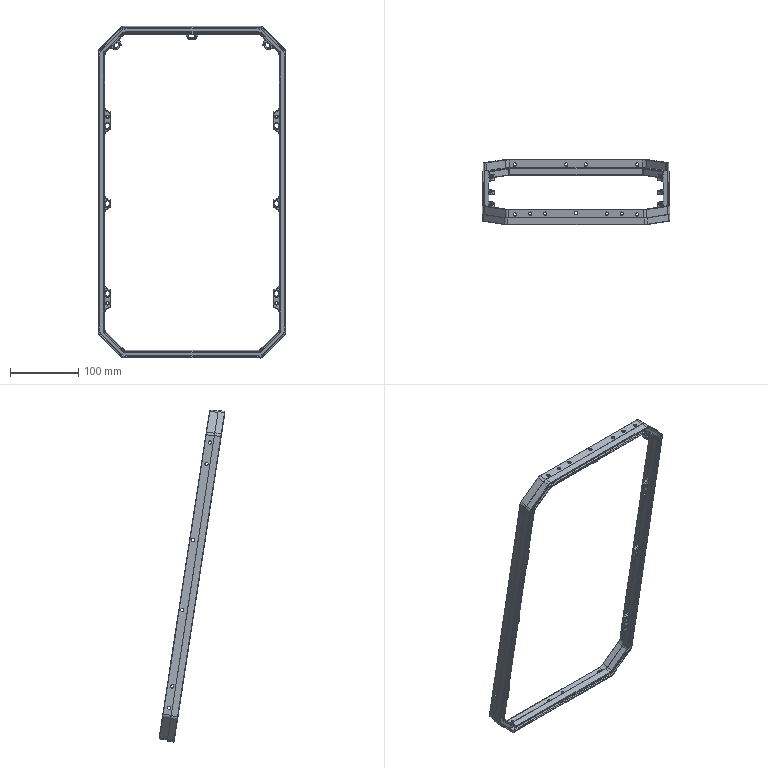Part | SolidWorks | features BaseBody 1 | 1 solid | 674 faces | box 275 x 96.615 x 486.269 mm | volume 140829 mm3 | cylinder 305 | plane 169 | torus 112 | spline 48 | cone 40 | commonest cylinder face diameters 2 x107 4.9 x46 8 x27 5.002 x21 1 x20 4 x20